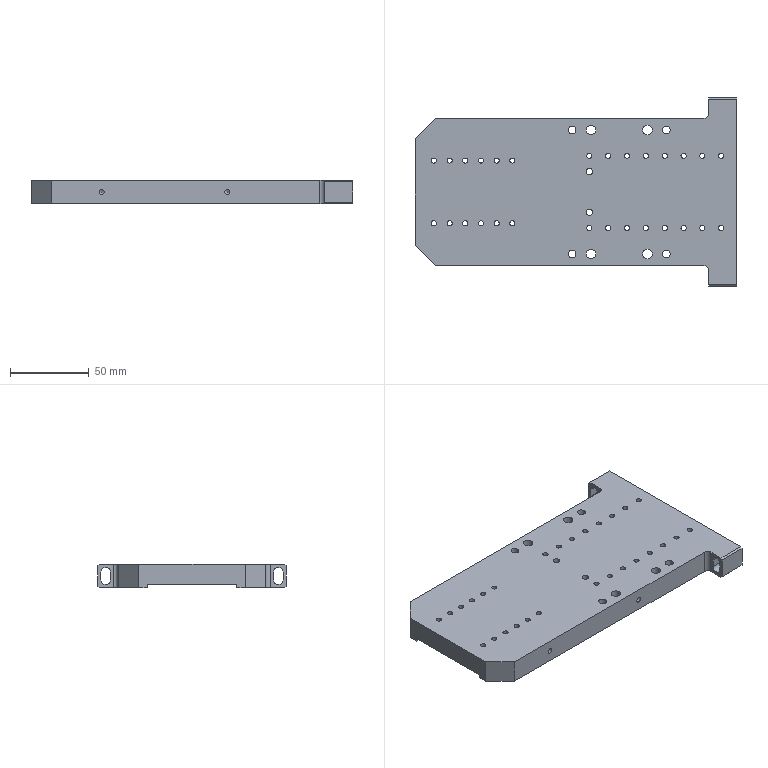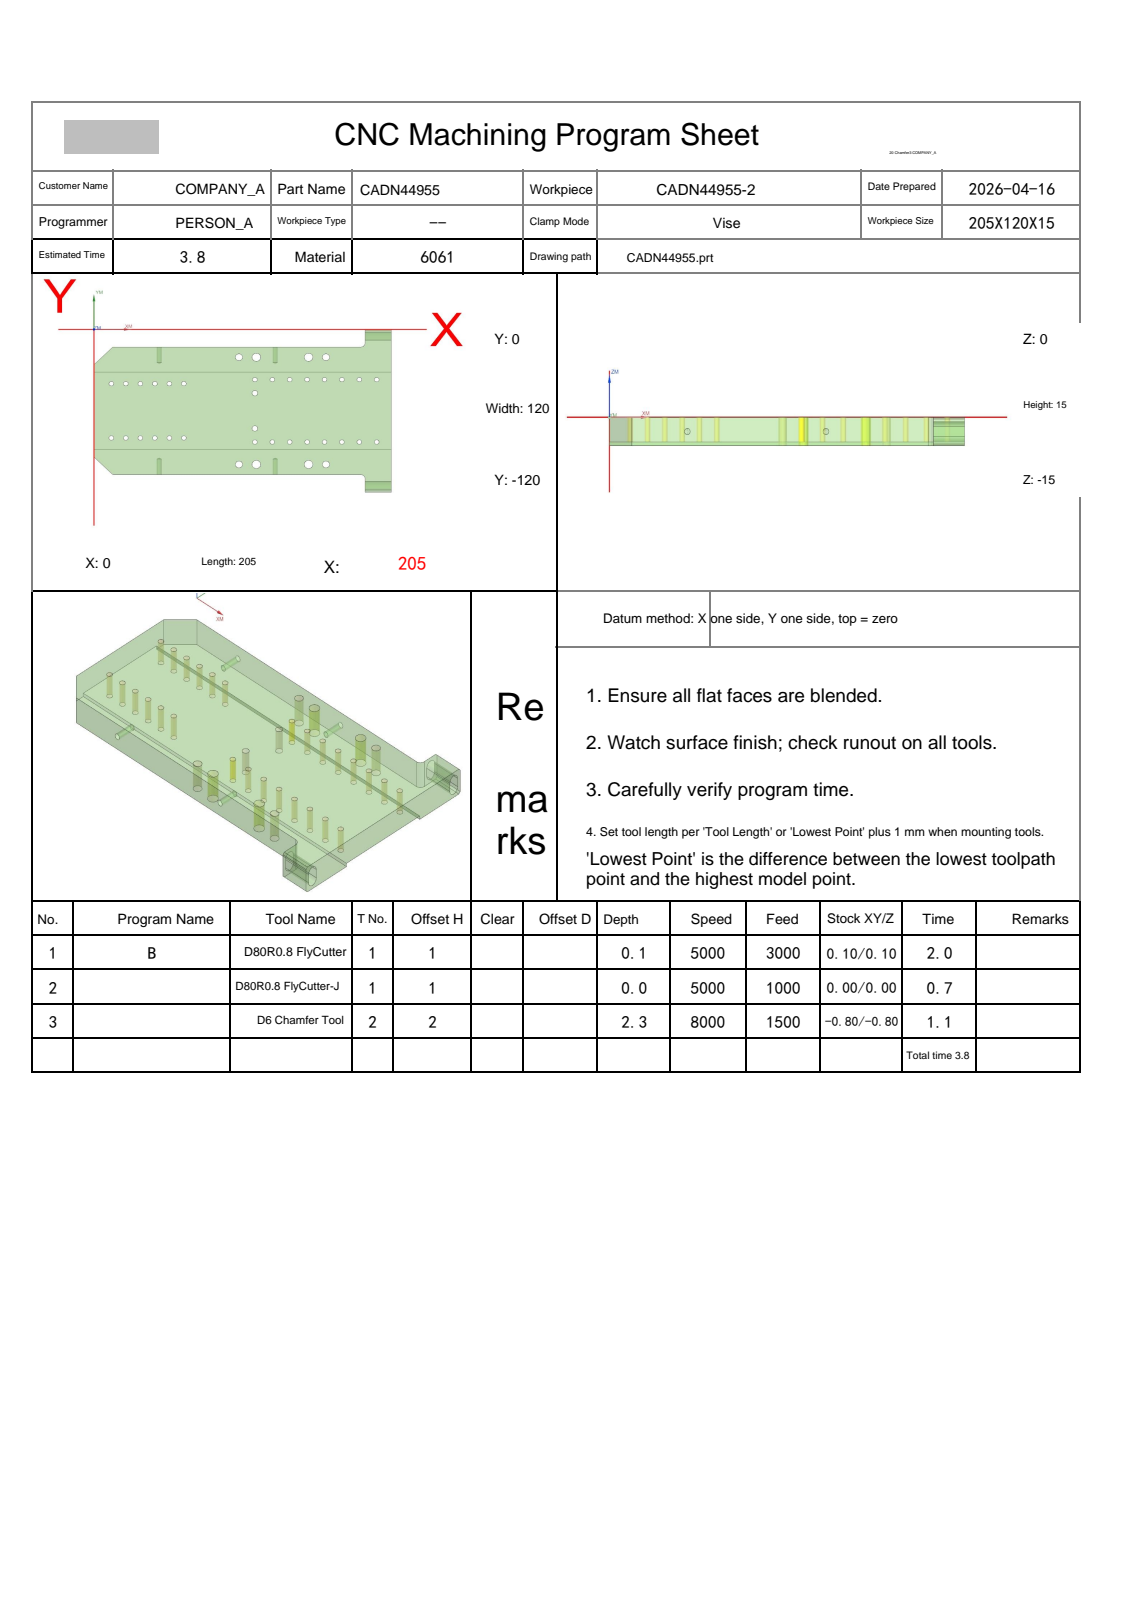NC program | NX | posted by the shop | part box 205 x 120 x 15 mm
Whole program:
%
O0001
(Machine time: 4.33 MIN)
(===Total Tool:2===)
(T1=D80R0.8 FlyCutter D=80.  R=0.8  D-  H01 Z=0.    )
(T2=D6 ChamferTool   D=6.   R=0.   D-  H02 Z=-2.3  )
G80 G90 G17 G49 G40
G91 G28 Z0
M01
N1 T01 M06
(D80R0.8 FlyCutter  D=80. R=0.8 H=01 ce=0.10 di=0.10)
G00 G90 G54 X-52.097 Y-23.903 M03 S5000
G43 H01 Z50.
M08
Z6.011
G01 Z4.011 F3000.
X-40.097
X237.1
G02 X245.097 Y-31.9 I-.003 J-8.
G01 Y-80.74
G02 X237.1 Y-88.737 I-8. J.004
G01 X-40.097
X-52.097
Z6.011
G00 Y-23.903
Z5.522
G01 Z3.522
X-40.097
X237.1
G02 X245.097 Y-31.9 I-.003 J-8.
G01 Y-80.74
G02 X237.1 Y-88.737 I-8. J.004
G01 X-40.097
X-52.097
Z5.522
G00 Y-23.903
Z5.033
G01 Z3.033
X-40.097
X237.1
G02 X245.097 Y-31.9 I-.003 J-8.
G01 Y-80.74
G02 X237.1 Y-88.737 I-8. J.004
G01 X-40.097
X-52.097
Z5.033
G00 Y-23.903
Z4.544
G01 Z2.544
X-40.097
X237.1
G02 X245.097 Y-31.9 I-.003 J-8.
G01 Y-80.74
G02 X237.1 Y-88.737 I-8. J.004
G01 X-40.097
X-52.097
Z4.544
G00 Y-23.903
Z4.056
G01 Z2.056
X-40.097
X237.1
G02 X245.097 Y-31.9 I-.003 J-8.
G01 Y-80.74
G02 X237.1 Y-88.737 I-8. J.004
G01 X-40.097
X-52.097
Z4.056
G00 Y-23.903
Z3.567
G01 Z1.567
X-40.097
X237.1
G02 X245.097 Y-31.9 I-.003 J-8.
G01 Y-80.74
G02 X237.1 Y-88.737 I-8. J.004
G01 X-40.097
X-52.097
Z3.567
G00 Y-23.903
Z3.078
G01 Z1.078
X-40.097
X237.1
G02 X245.097 Y-31.9 I-.003 J-8.
G01 Y-80.74
G02 X237.1 Y-88.737 I-8. J.004
G01 X-40.097
X-52.097
Z3.078
G00 Y-23.903
Z2.589
G01 Z.589
X-40.097
X237.1
G02 X245.097 Y-31.9 I-.003 J-8.
G01 Y-80.74
G02 X237.1 Y-88.737 I-8. J.004
G01 X-40.097
X-52.097
Z2.589
G00 Y-23.903
Z2.1
G01 Z.1
X-40.097
X237.1
G02 X245.097 Y-31.9 I-.003 J-8.
G01 Y-80.74
G02 X237.1 Y-88.737 I-8. J.004
G01 X-40.097
X-52.097
Z2.1
G00 Z50.
G91 G28 Z0.0
M05
M09
G91 G28 Z0.0
M01
N2 T01 M06
(D80R0.8 FlyCutter-J  D=80. R=0.8 H=01 ce=0.00 di=0.00)
G00 G90 G54 X-51.999 Y-24.001 M03 S5000
G43 H01 Z50.
M08
Z2.
G01 Z0.0 F1000.
X-39.999
X237.002
G02 X244.999 Y-31.998 I-.003 J-8.
G01 Y-80.642
G02 X237.002 Y-88.639 I-8. J.004
G01 X-39.999
X-51.999
Z2.
G00 Z50.
G91 G28 Z0.0
M05
M09
G91 G28 Z0.0
M01
N3 T02 M06
(D6 ChamferTool  D=6. R=0. H=02 ce=0.00 di=0.00)
G00 G90 G54 X62. Y-40. M03 S8000
G43 H02 Z20.
M08
G98 G81 X62. Y-40. Z-2.2 R3. F1000.
X52.
X42.
X32.
X22.
X12.
Y-80.
X22.
X32.
X42.
X52.
X62.
X111. Y-83.
X123.
X135.
X147.
X159.
X171.
X183.
X195.
Y-37.
X183.
X171.
X159.
X147.
X135.
X123.
X111.
G80
G00 Z20.
G00 G90 X111. Y-73. M03 S8000
Z20.
G98 G81 X111. Y-73. Z-2.3 R3. F1000.
Y-47.
G80
G00 Z20.
G00 G90 X100.232 Y-100.37 M03 S8000
Z50.
Z-.9
G01 Z-1.4 F600.
X100.4 Y-101.
G03 X101.9 Y-99.5 I0.0 J1.5
X100. Y-97.6 I-1.9 J0.0
X98.1 Y-99.5 I0.0 J-1.9
X100. Y-101.4 I1.9 J0.0
X101.9 Y-99.5 I0.0 J1.9
X100.4 Y-98. I-1.5 J0.0
G01 X100.232 Y-98.63
Z-.9
G00 Z50.
X160.232 Y-100.37
Z-.9
G01 Z-1.4
X160.4 Y-101.
G03 X161.9 Y-99.5 I0.0 J1.5
X160. Y-97.6 I-1.9 J0.0
X158.1 Y-99.5 I0.0 J-1.9
X160. Y-101.4 I1.9 J0.0
X161.9 Y-99.5 I0.0 J1.9
X160.4 Y-98. I-1.5 J0.0
G01 X160.232 Y-98.63
Z-.9
G00 Z50.
Y-21.37
Z-.9
G01 Z-1.4
X160.4 Y-22.
G03 X161.9 Y-20.5 I0.0 J1.5
X160. Y-18.6 I-1.9 J0.0
X158.1 Y-20.5 I0.0 J-1.9
X160. Y-22.4 I1.9 J0.0
X161.9 Y-20.5 I0.0 J1.9
X160.4 Y-19. I-1.5 J0.0
G01 X160.232 Y-19.63
Z-.9
G00 Z50.
X100.232 Y-21.37
Z-.9
G01 Z-1.4
X100.4 Y-22.
G03 X101.9 Y-20.5 I0.0 J1.5
X100. Y-18.6 I-1.9 J0.0
X98.1 Y-20.5 I0.0 J-1.9
X100. Y-22.4 I1.9 J0.0
X101.9 Y-20.5 I0.0 J1.9
X100.4 Y-19. I-1.5 J0.0
G01 X100.232 Y-19.63
Z-.9
G00 Z50.
G00 G90 X148.232 Y-21.37 M03 S8000
Z50.
Z-.9
G01 Z-1.4 F600.
X148.4 Y-22.
G03 X149.9 Y-20.5 I0.0 J1.5
X148. Y-18.6 I-1.9 J0.0
X146.1 Y-20.5 I0.0 J-1.9
X148. Y-22.4 I1.9 J0.0
X149.9 Y-20.5 I0.0 J1.9
X148.4 Y-19. I-1.5 J0.0
G01 X148.232 Y-19.63
Z-.9
G00 Z50.
X112.232 Y-21.37
Z-.9
G01 Z-1.4
X112.4 Y-22.
G03 X113.9 Y-20.5 I0.0 J1.5
X112. Y-18.6 I-1.9 J0.0
X110.1 Y-20.5 I0.0 J-1.9
X112. Y-22.4 I1.9 J0.0
X113.9 Y-20.5 I0.0 J1.9
X112.4 Y-19. I-1.5 J0.0
G01 X112.232 Y-19.63
Z-.9
G00 Z50.
Y-100.37
Z-.9
G01 Z-1.4
X112.4 Y-101.
G03 X113.9 Y-99.5 I0.0 J1.5
X112. Y-97.6 I-1.9 J0.0
X110.1 Y-99.5 I0.0 J-1.9
X112. Y-101.4 I1.9 J0.0
X113.9 Y-99.5 I0.0 J1.9
X112.4 Y-98. I-1.5 J0.0
G01 X112.232 Y-98.63
Z-.9
G00 Z50.
X148.232 Y-100.37
Z-.9
G01 Z-1.4
X148.4 Y-101.
G03 X149.9 Y-99.5 I0.0 J1.5
X148. Y-97.6 I-1.9 J0.0
X146.1 Y-99.5 I0.0 J-1.9
X148. Y-101.4 I1.9 J0.0
X149.9 Y-99.5 I0.0 J1.9
X148.4 Y-98. I-1.5 J0.0
G01 X148.232 Y-98.63
Z-.9
G00 Z50.
G00 G90 X205.7 Y-109.384 M03 S7000
Z50.
Z2.5
G01 Y-119. Z-1. F1500.
Y-119.7
G02 X204.7 Y-120.7 I-1. J0.0
G01 X187.3
G02 X186.3 Y-119.7 I0.0 J1.
G01 Y-110.
G03 X184. Y-107.7 I-2.3 J0.0
G01 X13.124
G02 X12.417 Y-107.407 I0.0 J1.
G01 X-.407 Y-94.583
G02 X-.7 Y-93.876 I.707 J.707
G01 Y-26.124
G02 X-.407 Y-25.417 I1. J0.0
G01 X12.417 Y-12.593
G02 X13.124 Y-12.3 I.707 J-.707
G01 X184.
G03 X186.3 Y-10. I0.0 J2.3
G01 Y-.3
G02 X187.3 Y.7 I1. J0.0
G01 X204.7
G02 X205.7 Y-.3 I0.0 J-1.
G01 Y-119.
Y-119.5
Z1.5
G00 Z50.
G00 G90 X184.1 Y.708 M03 S6500
Z50.
Z-.2
G01 Z-1.7 F1500.
X184.168 Y.699
X184.237 Y.7
X207.763
X207.832 Y.699
X207.9 Y.708
Z-.2
G00 Z50.
Y-120.708
Z-.2
G01 Z-1.7
X207.832 Y-120.699
X207.763 Y-120.7
X184.237
X184.168 Y-120.699
X184.1 Y-120.708
Z-.2
G00 Z50.
M05
M09
G91 G28 Z0.0
G91 G28 Y0.0
M30
%